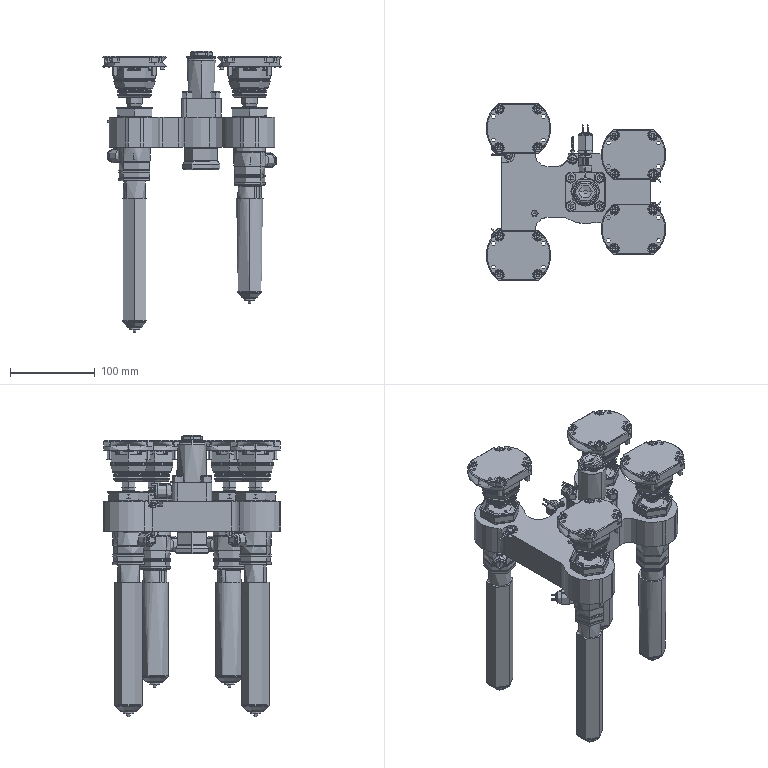Part | Creo | 1 solid | 3783 faces | volume 68266666666683453758449962001955305319044997064192953288065348355838929745159882927151099180484657152 mm3 | cylinder 1181 | plane 995 | torus 921 | cone 670 | spline 8 | sphere 6 | other 2 | commonest cylinder face diameters 6 x68 5 x52 6.5 x48 4 x43 10 x42 11 x42